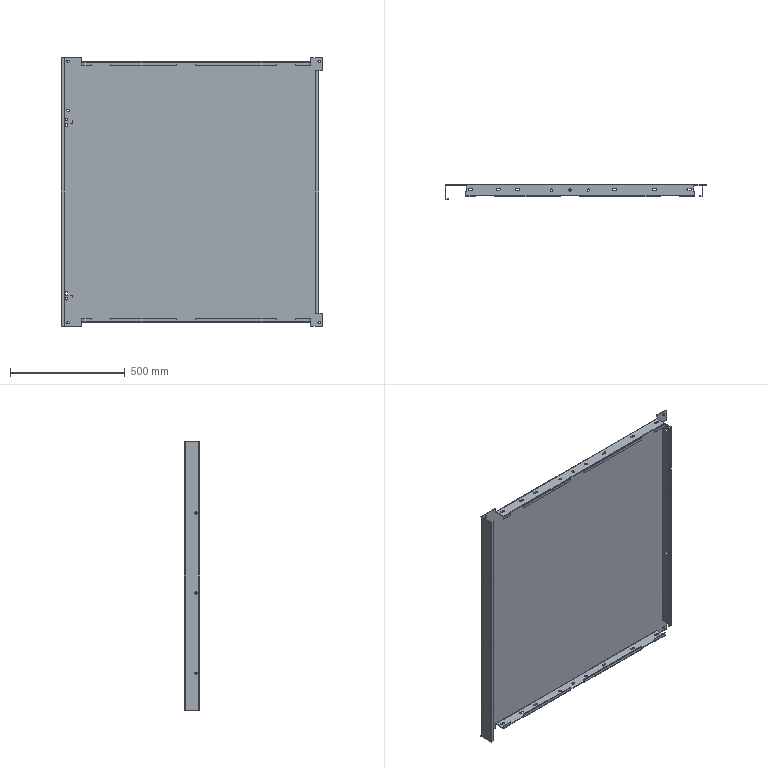Part | SolidWorks | features ICE 14, EdgeFlange 5, SMBaseFlange 3, Cut 2, Fillet 1, FlatPattern 1, MirrorPattern 1, SheetMetal 1 | 1 solid | 320 faces | box 1143 x 67 x 1171 mm | volume 4628360 mm3 | plane 206 | cylinder 114 | commonest cylinder face diameters 9 x36 10.5 x28 0.4 x14 6.4 x14 10 x14 6 x8